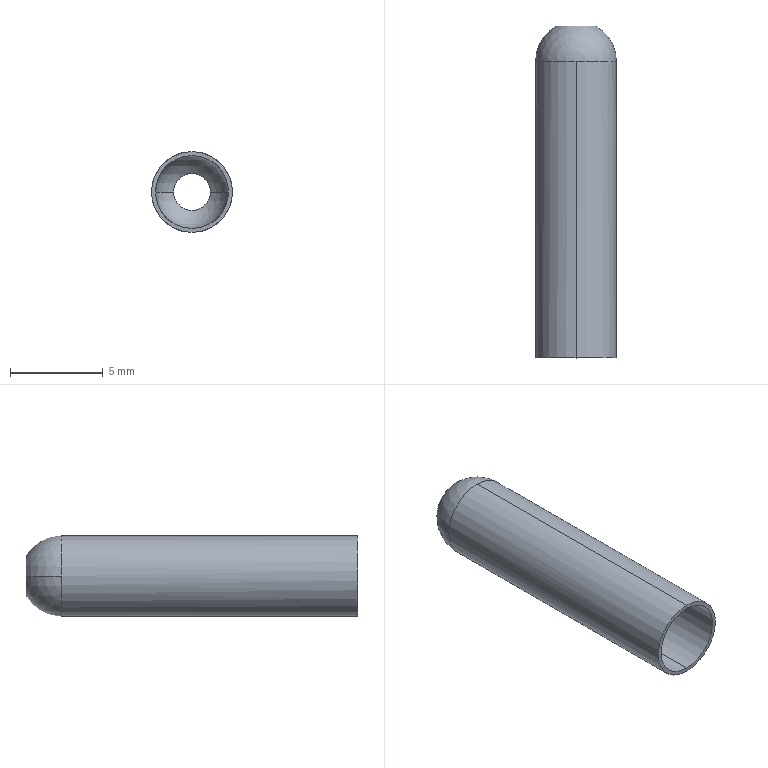Part | SolidWorks | features Revolution 1 | 1 solid | 12 faces | box 4.36 x 17.91 x 4.36 mm | volume 48.792 mm3 | cylinder 6 | sphere 4 | plane 2 | commonest cylinder face diameters 1.989 x2 3.94 x2 4.36 x2
STEP:
#1=CARTESIAN_POINT('',(0.,16.,1.97));
#2=VERTEX_POINT('',#1);
#3=CARTESIAN_POINT('',(-1.97,16.,0.));
#4=VERTEX_POINT('',#3);
#5=CARTESIAN_POINT('',(0.,16.,0.));
#6=DIRECTION('',(0.,-1.,0.));
#7=DIRECTION('',(0.,0.,-1.));
#8=AXIS2_PLACEMENT_3D('',#5,#6,#7);
#9=CIRCLE('',#8,1.97);
#10=EDGE_CURVE('',#2,#4,#9,.T.);
#11=ORIENTED_EDGE('',*,*,#10,.F.);
#12=CARTESIAN_POINT('',(0.,0.,1.97));
#13=VERTEX_POINT('',#12);
#14=CARTESIAN_POINT('',(0.,0.,1.97));
#15=DIRECTION('',(0.,-1.,0.));
#16=VECTOR('',#15,1000.);
#17=LINE('',#14,#16);
#18=EDGE_CURVE('',#2,#13,#17,.T.);
#19=ORIENTED_EDGE('',*,*,#18,.T.);
#20=CARTESIAN_POINT('',(0.,0.,-1.97));
#21=VERTEX_POINT('',#20);
#22=CARTESIAN_POINT('',(0.,0.,0.));
#23=DIRECTION('',(0.,-1.,0.));
#24=DIRECTION('',(0.,0.,-1.));
#25=AXIS2_PLACEMENT_3D('',#22,#23,#24);
#26=CIRCLE('',#25,1.97);
#27=EDGE_CURVE('',#13,#21,#26,.T.);
#28=ORIENTED_EDGE('',*,*,#27,.T.);
#29=CARTESIAN_POINT('',(0.,16.,-1.97));
#30=VERTEX_POINT('',#29);
#31=CARTESIAN_POINT('',(0.,0.,-1.97));
#32=DIRECTION('',(0.,-1.,0.));
#33=VECTOR('',#32,1000.);
#34=LINE('',#31,#33);
#35=EDGE_CURVE('',#30,#21,#34,.T.);
#36=ORIENTED_EDGE('',*,*,#35,.F.);
#37=CARTESIAN_POINT('',(0.,16.,0.));
#38=DIRECTION('',(0.,-1.,0.));
#39=DIRECTION('',(0.,0.,-1.));
#40=AXIS2_PLACEMENT_3D('',#37,#38,#39);
#41=CIRCLE('',#40,1.97);
#42=EDGE_CURVE('',#4,#30,#41,.T.);
#43=ORIENTED_EDGE('',*,*,#42,.F.);
#44=EDGE_LOOP('',(#11,#19,#28,#36,#43));
#45=FACE_OUTER_BOUND('',#44,.T.);
#46=CARTESIAN_POINT('',(0.,0.,0.));
#47=DIRECTION('',(0.,-1.,0.));
#48=DIRECTION('',(0.,0.,-1.));
#49=AXIS2_PLACEMENT_3D('',#46,#47,#48);
#50=CYLINDRICAL_SURFACE('',#49,1.97);
#51=ADVANCED_FACE('',(#45),#50,.F.);
#52=CARTESIAN_POINT('',(0.9946,17.7,0.));
#53=VERTEX_POINT('',#52);
#54=CARTESIAN_POINT('',(0.,17.7,0.9946));
#55=VERTEX_POINT('',#54);
#56=CARTESIAN_POINT('',(0.,17.7,0.));
#57=DIRECTION('',(0.,-1.,0.));
#58=DIRECTION('',(0.,0.,-1.));
#59=AXIS2_PLACEMENT_3D('',#56,#57,#58);
#60=CIRCLE('',#59,0.9946);
#61=EDGE_CURVE('',#53,#55,#60,.T.);
#62=ORIENTED_EDGE('',*,*,#61,.F.);
#63=CARTESIAN_POINT('',(1.97,16.,0.));
#64=VERTEX_POINT('',#63);
#65=CARTESIAN_POINT('',(0.,16.,0.));
#66=DIRECTION('',(0.,0.,-1.));
#67=DIRECTION('',(-1.,0.,0.));
#68=AXIS2_PLACEMENT_3D('',#65,#66,#67);
#69=CIRCLE('',#68,1.97);
#70=EDGE_CURVE('',#53,#64,#69,.T.);
#71=ORIENTED_EDGE('',*,*,#70,.T.);
#72=CARTESIAN_POINT('',(0.,16.,0.));
#73=DIRECTION('',(0.,-1.,0.));
#74=DIRECTION('',(0.,0.,-1.));
#75=AXIS2_PLACEMENT_3D('',#72,#73,#74);
#76=CIRCLE('',#75,1.97);
#77=EDGE_CURVE('',#64,#2,#76,.T.);
#78=ORIENTED_EDGE('',*,*,#77,.T.);
#79=ORIENTED_EDGE('',*,*,#10,.T.);
#80=CARTESIAN_POINT('',(-0.9946,17.7,0.));
#81=VERTEX_POINT('',#80);
#82=CARTESIAN_POINT('',(0.,16.,0.));
#83=DIRECTION('',(0.,0.,1.));
#84=DIRECTION('',(1.,0.,0.));
#85=AXIS2_PLACEMENT_3D('',#82,#83,#84);
#86=CIRCLE('',#85,1.97);
#87=EDGE_CURVE('',#81,#4,#86,.T.);
#88=ORIENTED_EDGE('',*,*,#87,.F.);
#89=CARTESIAN_POINT('',(0.,17.7,0.));
#90=DIRECTION('',(0.,-1.,0.));
#91=DIRECTION('',(0.,0.,-1.));
#92=AXIS2_PLACEMENT_3D('',#89,#90,#91);
#93=CIRCLE('',#92,0.9946);
#94=EDGE_CURVE('',#55,#81,#93,.T.);
#95=ORIENTED_EDGE('',*,*,#94,.F.);
#96=EDGE_LOOP('',(#62,#71,#78,#79,#88,#95));
#97=FACE_OUTER_BOUND('',#96,.T.);
#98=CARTESIAN_POINT('',(0.,16.,0.));
#99=DIRECTION('',(0.,0.,-1.));
#100=DIRECTION('',(-1.,0.,0.));
#101=AXIS2_PLACEMENT_3D('',#98,#99,#100);
#102=SPHERICAL_SURFACE('',#101,1.97);
#103=ADVANCED_FACE('',(#97),#102,.F.);
#104=CARTESIAN_POINT('',(0.,17.91,0.9946));
#105=VERTEX_POINT('',#104);
#106=CARTESIAN_POINT('',(0.,17.91,-0.9946));
#107=VERTEX_POINT('',#106);
#108=CARTESIAN_POINT('',(0.,17.91,0.));
#109=DIRECTION('',(0.,-1.,0.));
#110=DIRECTION('',(0.,0.,-1.));
#111=AXIS2_PLACEMENT_3D('',#108,#109,#110);
#112=CIRCLE('',#111,0.9946);
#113=EDGE_CURVE('',#105,#107,#112,.T.);
#114=ORIENTED_EDGE('',*,*,#113,.F.);
#115=CARTESIAN_POINT('',(0.,0.,0.9946));
#116=DIRECTION('',(0.,-1.,0.));
#117=VECTOR('',#116,1000.);
#118=LINE('',#115,#117);
#119=EDGE_CURVE('',#105,#55,#118,.T.);
#120=ORIENTED_EDGE('',*,*,#119,.T.);
#121=ORIENTED_EDGE('',*,*,#94,.T.);
#122=CARTESIAN_POINT('',(0.,17.7,-0.9946));
#123=VERTEX_POINT('',#122);
#124=CARTESIAN_POINT('',(0.,17.7,0.));
#125=DIRECTION('',(0.,-1.,0.));
#126=DIRECTION('',(0.,0.,-1.));
#127=AXIS2_PLACEMENT_3D('',#124,#125,#126);
#128=CIRCLE('',#127,0.9946);
#129=EDGE_CURVE('',#81,#123,#128,.T.);
#130=ORIENTED_EDGE('',*,*,#129,.T.);
#131=CARTESIAN_POINT('',(0.,0.,-0.9946));
#132=DIRECTION('',(0.,-1.,0.));
#133=VECTOR('',#132,1000.);
#134=LINE('',#131,#133);
#135=EDGE_CURVE('',#107,#123,#134,.T.);
#136=ORIENTED_EDGE('',*,*,#135,.F.);
#137=EDGE_LOOP('',(#114,#120,#121,#130,#136));
#138=FACE_OUTER_BOUND('',#137,.T.);
#139=CARTESIAN_POINT('',(0.,0.,0.));
#140=DIRECTION('',(0.,-1.,0.));
#141=DIRECTION('',(0.,0.,-1.));
#142=AXIS2_PLACEMENT_3D('',#139,#140,#141);
#143=CYLINDRICAL_SURFACE('',#142,0.9946);
#144=ADVANCED_FACE('',(#138),#143,.F.);
#145=CARTESIAN_POINT('',(-1.05,17.91,0.));
#146=VERTEX_POINT('',#145);
#147=CARTESIAN_POINT('',(1.05,17.91,0.));
#148=VERTEX_POINT('',#147);
#149=CARTESIAN_POINT('',(0.,17.91,0.));
#150=DIRECTION('',(0.,-1.,0.));
#151=DIRECTION('',(0.,0.,-1.));
#152=AXIS2_PLACEMENT_3D('',#149,#150,#151);
#153=CIRCLE('',#152,1.05);
#154=EDGE_CURVE('',#146,#148,#153,.T.);
#155=ORIENTED_EDGE('',*,*,#154,.T.);
#156=CARTESIAN_POINT('',(2.18,16.,0.));
#157=VERTEX_POINT('',#156);
#158=CARTESIAN_POINT('',(0.,16.,0.));
#159=DIRECTION('',(0.,0.,-1.));
#160=DIRECTION('',(-1.,0.,0.));
#161=AXIS2_PLACEMENT_3D('',#158,#159,#160);
#162=CIRCLE('',#161,2.18);
#163=EDGE_CURVE('',#148,#157,#162,.T.);
#164=ORIENTED_EDGE('',*,*,#163,.T.);
#165=CARTESIAN_POINT('',(0.,16.,-2.18));
#166=VERTEX_POINT('',#165);
#167=CARTESIAN_POINT('',(0.,16.,0.));
#168=DIRECTION('',(0.,-1.,0.));
#169=DIRECTION('',(0.,0.,-1.));
#170=AXIS2_PLACEMENT_3D('',#167,#168,#169);
#171=CIRCLE('',#170,2.18);
#172=EDGE_CURVE('',#166,#157,#171,.T.);
#173=ORIENTED_EDGE('',*,*,#172,.F.);
#174=CARTESIAN_POINT('',(-2.18,16.,0.));
#175=VERTEX_POINT('',#174);
#176=CARTESIAN_POINT('',(0.,16.,0.));
#177=DIRECTION('',(0.,-1.,0.));
#178=DIRECTION('',(0.,0.,-1.));
#179=AXIS2_PLACEMENT_3D('',#176,#177,#178);
#180=CIRCLE('',#179,2.18);
#181=EDGE_CURVE('',#175,#166,#180,.T.);
#182=ORIENTED_EDGE('',*,*,#181,.F.);
#183=CARTESIAN_POINT('',(0.,16.,0.));
#184=DIRECTION('',(0.,0.,1.));
#185=DIRECTION('',(1.,0.,0.));
#186=AXIS2_PLACEMENT_3D('',#183,#184,#185);
#187=CIRCLE('',#186,2.18);
#188=EDGE_CURVE('',#146,#175,#187,.T.);
#189=ORIENTED_EDGE('',*,*,#188,.F.);
#190=EDGE_LOOP('',(#155,#164,#173,#182,#189));
#191=FACE_OUTER_BOUND('',#190,.T.);
#192=CARTESIAN_POINT('',(0.,16.,0.));
#193=DIRECTION('',(0.,0.,-1.));
#194=DIRECTION('',(-1.,0.,0.));
#195=AXIS2_PLACEMENT_3D('',#192,#193,#194);
#196=SPHERICAL_SURFACE('',#195,2.18);
#197=ADVANCED_FACE('',(#191),#196,.T.);
#198=ORIENTED_EDGE('',*,*,#172,.T.);
#199=CARTESIAN_POINT('',(0.,16.,2.18));
#200=VERTEX_POINT('',#199);
#201=CARTESIAN_POINT('',(0.,16.,0.));
#202=DIRECTION('',(0.,-1.,0.));
#203=DIRECTION('',(0.,0.,-1.));
#204=AXIS2_PLACEMENT_3D('',#201,#202,#203);
#205=CIRCLE('',#204,2.18);
#206=EDGE_CURVE('',#157,#200,#205,.T.);
#207=ORIENTED_EDGE('',*,*,#206,.T.);
#208=CARTESIAN_POINT('',(0.,0.,2.18));
#209=VERTEX_POINT('',#208);
#210=CARTESIAN_POINT('',(0.,0.,2.18));
#211=DIRECTION('',(0.,-1.,0.));
#212=VECTOR('',#211,1000.);
#213=LINE('',#210,#212);
#214=EDGE_CURVE('',#200,#209,#213,.T.);
#215=ORIENTED_EDGE('',*,*,#214,.T.);
#216=CARTESIAN_POINT('',(0.,0.,-2.18));
#217=VERTEX_POINT('',#216);
#218=CARTESIAN_POINT('',(0.,0.,0.));
#219=DIRECTION('',(0.,-1.,0.));
#220=DIRECTION('',(0.,0.,-1.));
#221=AXIS2_PLACEMENT_3D('',#218,#219,#220);
#222=CIRCLE('',#221,2.18);
#223=EDGE_CURVE('',#217,#209,#222,.T.);
#224=ORIENTED_EDGE('',*,*,#223,.F.);
#225=CARTESIAN_POINT('',(0.,0.,-2.18));
#226=DIRECTION('',(0.,-1.,0.));
#227=VECTOR('',#226,1000.);
#228=LINE('',#225,#227);
#229=EDGE_CURVE('',#166,#217,#228,.T.);
#230=ORIENTED_EDGE('',*,*,#229,.F.);
#231=EDGE_LOOP('',(#198,#207,#215,#224,#230));
#232=FACE_OUTER_BOUND('',#231,.T.);
#233=CARTESIAN_POINT('',(0.,0.,0.));
#234=DIRECTION('',(0.,-1.,0.));
#235=DIRECTION('',(0.,0.,-1.));
#236=AXIS2_PLACEMENT_3D('',#233,#234,#235);
#237=CYLINDRICAL_SURFACE('',#236,2.18);
#238=ADVANCED_FACE('',(#232),#237,.T.);
#239=CARTESIAN_POINT('',(0.,0.,0.));
#240=DIRECTION('',(0.,-1.,0.));
#241=DIRECTION('',(0.,0.,-1.));
#242=AXIS2_PLACEMENT_3D('',#239,#240,#241);
#243=CIRCLE('',#242,1.97);
#244=EDGE_CURVE('',#21,#13,#243,.T.);
#245=ORIENTED_EDGE('',*,*,#244,.F.);
#246=ORIENTED_EDGE('',*,*,#27,.F.);
#247=EDGE_LOOP('',(#245,#246));
#248=FACE_BOUND('',#247,.T.);
#249=ORIENTED_EDGE('',*,*,#223,.T.);
#250=CARTESIAN_POINT('',(0.,0.,0.));
#251=DIRECTION('',(0.,-1.,0.));
#252=DIRECTION('',(0.,0.,-1.));
#253=AXIS2_PLACEMENT_3D('',#250,#251,#252);
#254=CIRCLE('',#253,2.18);
#255=EDGE_CURVE('',#209,#217,#254,.T.);
#256=ORIENTED_EDGE('',*,*,#255,.T.);
#257=EDGE_LOOP('',(#249,#256));
#258=FACE_OUTER_BOUND('',#257,.T.);
#259=CARTESIAN_POINT('',(-2.18,0.,0.));
#260=DIRECTION('',(0.,1.,0.));
#261=DIRECTION('',(0.,0.,1.));
#262=AXIS2_PLACEMENT_3D('',#259,#260,#261);
#263=PLANE('',#262);
#264=ADVANCED_FACE('',(#248,#258),#263,.F.);
#265=ORIENTED_EDGE('',*,*,#214,.F.);
#266=CARTESIAN_POINT('',(0.,16.,0.));
#267=DIRECTION('',(0.,-1.,0.));
#268=DIRECTION('',(0.,0.,-1.));
#269=AXIS2_PLACEMENT_3D('',#266,#267,#268);
#270=CIRCLE('',#269,2.18);
#271=EDGE_CURVE('',#200,#175,#270,.T.);
#272=ORIENTED_EDGE('',*,*,#271,.T.);
#273=ORIENTED_EDGE('',*,*,#181,.T.);
#274=ORIENTED_EDGE('',*,*,#229,.T.);
#275=ORIENTED_EDGE('',*,*,#255,.F.);
#276=EDGE_LOOP('',(#265,#272,#273,#274,#275));
#277=FACE_OUTER_BOUND('',#276,.T.);
#278=CARTESIAN_POINT('',(0.,0.,0.));
#279=DIRECTION('',(0.,-1.,0.));
#280=DIRECTION('',(0.,0.,-1.));
#281=AXIS2_PLACEMENT_3D('',#278,#279,#280);
#282=CYLINDRICAL_SURFACE('',#281,2.18);
#283=ADVANCED_FACE('',(#277),#282,.T.);
#284=ORIENTED_EDGE('',*,*,#163,.F.);
#285=CARTESIAN_POINT('',(0.,17.91,0.));
#286=DIRECTION('',(0.,-1.,0.));
#287=DIRECTION('',(0.,0.,-1.));
#288=AXIS2_PLACEMENT_3D('',#285,#286,#287);
#289=CIRCLE('',#288,1.05);
#290=EDGE_CURVE('',#148,#146,#289,.T.);
#291=ORIENTED_EDGE('',*,*,#290,.T.);
#292=ORIENTED_EDGE('',*,*,#188,.T.);
#293=ORIENTED_EDGE('',*,*,#271,.F.);
#294=ORIENTED_EDGE('',*,*,#206,.F.);
#295=EDGE_LOOP('',(#284,#291,#292,#293,#294));
#296=FACE_OUTER_BOUND('',#295,.T.);
#297=CARTESIAN_POINT('',(0.,16.,0.));
#298=DIRECTION('',(0.,0.,-1.));
#299=DIRECTION('',(-1.,0.,0.));
#300=AXIS2_PLACEMENT_3D('',#297,#298,#299);
#301=SPHERICAL_SURFACE('',#300,2.18);
#302=ADVANCED_FACE('',(#296),#301,.T.);
#303=ORIENTED_EDGE('',*,*,#154,.F.);
#304=ORIENTED_EDGE('',*,*,#290,.F.);
#305=EDGE_LOOP('',(#303,#304));
#306=FACE_OUTER_BOUND('',#305,.T.);
#307=CARTESIAN_POINT('',(0.,17.91,0.));
#308=DIRECTION('',(0.,-1.,0.));
#309=DIRECTION('',(0.,0.,-1.));
#310=AXIS2_PLACEMENT_3D('',#307,#308,#309);
#311=CIRCLE('',#310,0.9946);
#312=EDGE_CURVE('',#107,#105,#311,.T.);
#313=ORIENTED_EDGE('',*,*,#312,.T.);
#314=ORIENTED_EDGE('',*,*,#113,.T.);
#315=EDGE_LOOP('',(#313,#314));
#316=FACE_BOUND('',#315,.T.);
#317=CARTESIAN_POINT('',(-1.05,17.91,0.));
#318=DIRECTION('',(0.,-1.,0.));
#319=DIRECTION('',(0.,0.,-1.));
#320=AXIS2_PLACEMENT_3D('',#317,#318,#319);
#321=PLANE('',#320);
#322=ADVANCED_FACE('',(#306,#316),#321,.F.);
#323=ORIENTED_EDGE('',*,*,#119,.F.);
#324=ORIENTED_EDGE('',*,*,#312,.F.);
#325=ORIENTED_EDGE('',*,*,#135,.T.);
#326=CARTESIAN_POINT('',(0.,17.7,0.));
#327=DIRECTION('',(0.,-1.,0.));
#328=DIRECTION('',(0.,0.,-1.));
#329=AXIS2_PLACEMENT_3D('',#326,#327,#328);
#330=CIRCLE('',#329,0.9946);
#331=EDGE_CURVE('',#123,#53,#330,.T.);
#332=ORIENTED_EDGE('',*,*,#331,.T.);
#333=ORIENTED_EDGE('',*,*,#61,.T.);
#334=EDGE_LOOP('',(#323,#324,#325,#332,#333));
#335=FACE_OUTER_BOUND('',#334,.T.);
#336=CARTESIAN_POINT('',(0.,0.,0.));
#337=DIRECTION('',(0.,-1.,0.));
#338=DIRECTION('',(0.,0.,-1.));
#339=AXIS2_PLACEMENT_3D('',#336,#337,#338);
#340=CYLINDRICAL_SURFACE('',#339,0.9946);
#341=ADVANCED_FACE('',(#335),#340,.F.);
#342=ORIENTED_EDGE('',*,*,#70,.F.);
#343=ORIENTED_EDGE('',*,*,#331,.F.);
#344=ORIENTED_EDGE('',*,*,#129,.F.);
#345=ORIENTED_EDGE('',*,*,#87,.T.);
#346=ORIENTED_EDGE('',*,*,#42,.T.);
#347=CARTESIAN_POINT('',(0.,16.,0.));
#348=DIRECTION('',(0.,-1.,0.));
#349=DIRECTION('',(0.,0.,-1.));
#350=AXIS2_PLACEMENT_3D('',#347,#348,#349);
#351=CIRCLE('',#350,1.97);
#352=EDGE_CURVE('',#30,#64,#351,.T.);
#353=ORIENTED_EDGE('',*,*,#352,.T.);
#354=EDGE_LOOP('',(#342,#343,#344,#345,#346,#353));
#355=FACE_OUTER_BOUND('',#354,.T.);
#356=CARTESIAN_POINT('',(0.,16.,0.));
#357=DIRECTION('',(0.,0.,-1.));
#358=DIRECTION('',(-1.,0.,0.));
#359=AXIS2_PLACEMENT_3D('',#356,#357,#358);
#360=SPHERICAL_SURFACE('',#359,1.97);
#361=ADVANCED_FACE('',(#355),#360,.F.);
#362=ORIENTED_EDGE('',*,*,#18,.F.);
#363=ORIENTED_EDGE('',*,*,#77,.F.);
#364=ORIENTED_EDGE('',*,*,#352,.F.);
#365=ORIENTED_EDGE('',*,*,#35,.T.);
#366=ORIENTED_EDGE('',*,*,#244,.T.);
#367=EDGE_LOOP('',(#362,#363,#364,#365,#366));
#368=FACE_OUTER_BOUND('',#367,.T.);
#369=CARTESIAN_POINT('',(0.,0.,0.));
#370=DIRECTION('',(0.,-1.,0.));
#371=DIRECTION('',(0.,0.,-1.));
#372=AXIS2_PLACEMENT_3D('',#369,#370,#371);
#373=CYLINDRICAL_SURFACE('',#372,1.97);
#374=ADVANCED_FACE('',(#368),#373,.F.);
#375=CLOSED_SHELL('',(#51,#103,#144,#197,#238,#264,#283,#302,#322,#341,#361,#374));
#376=MANIFOLD_SOLID_BREP('',#375);
#377=CARTESIAN_POINT('',(0.,0.,0.));
#378=DIRECTION('',(0.,0.,1.));
#379=DIRECTION('',(1.,0.,0.));
#380=AXIS2_PLACEMENT_3D('',#377,#378,#379);
#381=(LENGTH_UNIT()NAMED_UNIT(*)SI_UNIT(.MILLI.,.METRE.));
#382=UNCERTAINTY_MEASURE_WITH_UNIT(LENGTH_MEASURE(0.00001),#381,'','');
#383=(NAMED_UNIT(*)PLANE_ANGLE_UNIT()SI_UNIT($,.RADIAN.));
#384=(NAMED_UNIT(*)SI_UNIT($,.STERADIAN.)SOLID_ANGLE_UNIT());
#385=(GEOMETRIC_REPRESENTATION_CONTEXT(3)GLOBAL_UNCERTAINTY_ASSIGNED_CONTEXT((#382))GLOBAL_UNIT_ASSIGNED_CONTEXT((#381,#383,#384))REPRESENTATION_CONTEXT('',''));
#386=ADVANCED_BREP_SHAPE_REPRESENTATION('',(#376,#380),#385);